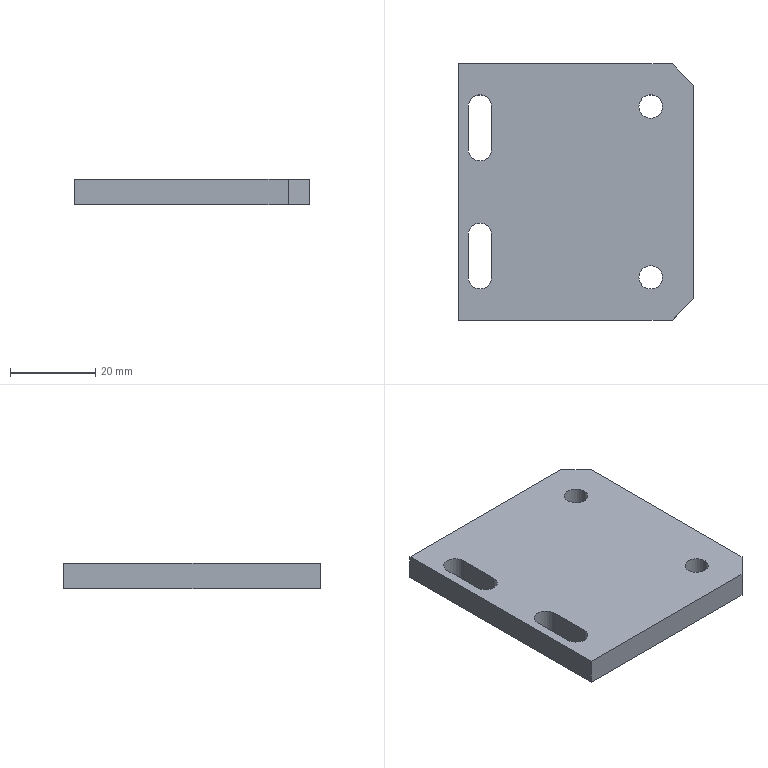Part | STEP file | 0232_206_Plate | 1 solid | 20 faces | box 55 x 60 x 6 mm | volume 18420 mm3 | plane 12 | cylinder 8 | commonest cylinder face diameters 5.5 x8
STEP:
#1=CARTESIAN_POINT('',(0.,0.,0.));
#2=DIRECTION('',(0.,0.,1.));
#3=DIRECTION('',(1.,0.,0.));
#4=AXIS2_PLACEMENT_3D('',#1,#2,#3);
#5=CARTESIAN_POINT('',(-7.25,-20.,0.));
#6=VERTEX_POINT('',#5);
#7=CARTESIAN_POINT('',(-7.25,-20.,6.));
#8=VERTEX_POINT('',#7);
#9=CARTESIAN_POINT('',(-7.25,-20.,6.));
#10=DIRECTION('',(0.,0.,1.));
#11=VECTOR('',#10,1.);
#12=LINE('',#9,#11);
#13=CARTESIAN_POINT('',(-10.,-20.,6.));
#14=DIRECTION('',(0.,0.,1.));
#15=DIRECTION('',(1.,0.,0.));
#16=AXIS2_PLACEMENT_3D('',#13,#14,#15);
#17=CYLINDRICAL_SURFACE('',#16,2.75);
#18=CARTESIAN_POINT('',(6.283,0.));
#19=DIRECTION('',(0.,1.));
#20=VECTOR('',#19,1.);
#21=LINE('',#18,#20);
#22=(GEOMETRIC_REPRESENTATION_CONTEXT(2)PARAMETRIC_REPRESENTATION_CONTEXT()REPRESENTATION_CONTEXT('',''));
#23=DEFINITIONAL_REPRESENTATION('',(#21),#22);
#24=PCURVE('',#17,#23);
#25=CARTESIAN_POINT('',(-10.,-20.,6.));
#26=DIRECTION('',(0.,0.,1.));
#27=DIRECTION('',(1.,0.,0.));
#28=AXIS2_PLACEMENT_3D('',#25,#26,#27);
#29=CYLINDRICAL_SURFACE('',#28,2.75);
#30=CARTESIAN_POINT('',(0.,0.));
#31=DIRECTION('',(0.,1.));
#32=VECTOR('',#31,1.);
#33=LINE('',#30,#32);
#34=(GEOMETRIC_REPRESENTATION_CONTEXT(2)PARAMETRIC_REPRESENTATION_CONTEXT()REPRESENTATION_CONTEXT('',''));
#35=DEFINITIONAL_REPRESENTATION('',(#33),#34);
#36=PCURVE('',#29,#35);
#37=SURFACE_CURVE('',#12,(#24,#36),.PCURVE_S1.);
#38=EDGE_CURVE('',#6,#8,#37,.T.);
#39=ORIENTED_EDGE('',*,*,#38,.T.);
#40=CARTESIAN_POINT('',(-12.75,-20.,6.));
#41=VERTEX_POINT('',#40);
#42=CARTESIAN_POINT('',(-10.,-20.,6.));
#43=DIRECTION('',(0.,0.,1.));
#44=DIRECTION('',(1.,0.,0.));
#45=AXIS2_PLACEMENT_3D('',#42,#43,#44);
#46=CIRCLE('',#45,2.75);
#47=CARTESIAN_POINT('',(0.,0.));
#48=DIRECTION('',(1.,0.));
#49=VECTOR('',#48,1.);
#50=LINE('',#47,#49);
#51=(GEOMETRIC_REPRESENTATION_CONTEXT(2)PARAMETRIC_REPRESENTATION_CONTEXT()REPRESENTATION_CONTEXT('',''));
#52=DEFINITIONAL_REPRESENTATION('',(#50),#51);
#53=PCURVE('',#17,#52);
#54=CARTESIAN_POINT('',(-55.,-30.,6.));
#55=DIRECTION('',(0.,0.,1.));
#56=DIRECTION('',(1.,0.,0.));
#57=AXIS2_PLACEMENT_3D('',#54,#55,#56);
#58=PLANE('',#57);
#59=CARTESIAN_POINT('',(45.,10.));
#60=DIRECTION('',(1.,0.));
#61=AXIS2_PLACEMENT_2D('',#59,#60);
#62=CIRCLE('',#61,2.75);
#63=(GEOMETRIC_REPRESENTATION_CONTEXT(2)PARAMETRIC_REPRESENTATION_CONTEXT()REPRESENTATION_CONTEXT('',''));
#64=DEFINITIONAL_REPRESENTATION('',(#62),#63);
#65=PCURVE('',#58,#64);
#66=SURFACE_CURVE('',#46,(#53,#65),.PCURVE_S1.);
#67=EDGE_CURVE('',#41,#8,#66,.T.);
#68=ORIENTED_EDGE('',*,*,#67,.F.);
#69=CARTESIAN_POINT('',(-12.75,-20.,0.));
#70=VERTEX_POINT('',#69);
#71=CARTESIAN_POINT('',(-12.75,-20.,6.));
#72=DIRECTION('',(0.,0.,1.));
#73=VECTOR('',#72,1.);
#74=LINE('',#71,#73);
#75=CARTESIAN_POINT('',(3.142,0.));
#76=DIRECTION('',(0.,1.));
#77=VECTOR('',#76,1.);
#78=LINE('',#75,#77);
#79=(GEOMETRIC_REPRESENTATION_CONTEXT(2)PARAMETRIC_REPRESENTATION_CONTEXT()REPRESENTATION_CONTEXT('',''));
#80=DEFINITIONAL_REPRESENTATION('',(#78),#79);
#81=PCURVE('',#17,#80);
#82=CARTESIAN_POINT('',(3.142,0.));
#83=DIRECTION('',(0.,1.));
#84=VECTOR('',#83,1.);
#85=LINE('',#82,#84);
#86=(GEOMETRIC_REPRESENTATION_CONTEXT(2)PARAMETRIC_REPRESENTATION_CONTEXT()REPRESENTATION_CONTEXT('',''));
#87=DEFINITIONAL_REPRESENTATION('',(#85),#86);
#88=PCURVE('',#29,#87);
#89=SURFACE_CURVE('',#74,(#81,#88),.PCURVE_S1.);
#90=EDGE_CURVE('',#70,#41,#89,.T.);
#91=ORIENTED_EDGE('',*,*,#90,.F.);
#92=CARTESIAN_POINT('',(-10.,-20.,0.));
#93=DIRECTION('',(0.,0.,1.));
#94=DIRECTION('',(1.,0.,0.));
#95=AXIS2_PLACEMENT_3D('',#92,#93,#94);
#96=CIRCLE('',#95,2.75);
#97=CARTESIAN_POINT('',(0.,-6.));
#98=DIRECTION('',(1.,0.));
#99=VECTOR('',#98,1.);
#100=LINE('',#97,#99);
#101=(GEOMETRIC_REPRESENTATION_CONTEXT(2)PARAMETRIC_REPRESENTATION_CONTEXT()REPRESENTATION_CONTEXT('',''));
#102=DEFINITIONAL_REPRESENTATION('',(#100),#101);
#103=PCURVE('',#17,#102);
#104=CARTESIAN_POINT('',(-55.,-30.,0.));
#105=DIRECTION('',(0.,0.,1.));
#106=DIRECTION('',(1.,0.,0.));
#107=AXIS2_PLACEMENT_3D('',#104,#105,#106);
#108=PLANE('',#107);
#109=CARTESIAN_POINT('',(45.,10.));
#110=DIRECTION('',(1.,0.));
#111=AXIS2_PLACEMENT_2D('',#109,#110);
#112=CIRCLE('',#111,2.75);
#113=(GEOMETRIC_REPRESENTATION_CONTEXT(2)PARAMETRIC_REPRESENTATION_CONTEXT()REPRESENTATION_CONTEXT('',''));
#114=DEFINITIONAL_REPRESENTATION('',(#112),#113);
#115=PCURVE('',#108,#114);
#116=SURFACE_CURVE('',#96,(#103,#115),.PCURVE_S1.);
#117=EDGE_CURVE('',#70,#6,#116,.T.);
#118=ORIENTED_EDGE('',*,*,#117,.T.);
#119=EDGE_LOOP('',(#39,#68,#91,#118));
#120=FACE_BOUND('',#119,.F.);
#121=ADVANCED_FACE('',(#120),#17,.F.);
#122=CARTESIAN_POINT('',(-7.25,20.,0.));
#123=VERTEX_POINT('',#122);
#124=CARTESIAN_POINT('',(-7.25,20.,6.));
#125=VERTEX_POINT('',#124);
#126=CARTESIAN_POINT('',(-7.25,20.,6.));
#127=DIRECTION('',(0.,0.,1.));
#128=VECTOR('',#127,1.);
#129=LINE('',#126,#128);
#130=CARTESIAN_POINT('',(-10.,20.,6.));
#131=DIRECTION('',(0.,0.,1.));
#132=DIRECTION('',(1.,0.,0.));
#133=AXIS2_PLACEMENT_3D('',#130,#131,#132);
#134=CYLINDRICAL_SURFACE('',#133,2.75);
#135=CARTESIAN_POINT('',(6.283,0.));
#136=DIRECTION('',(0.,1.));
#137=VECTOR('',#136,1.);
#138=LINE('',#135,#137);
#139=(GEOMETRIC_REPRESENTATION_CONTEXT(2)PARAMETRIC_REPRESENTATION_CONTEXT()REPRESENTATION_CONTEXT('',''));
#140=DEFINITIONAL_REPRESENTATION('',(#138),#139);
#141=PCURVE('',#134,#140);
#142=CARTESIAN_POINT('',(-10.,20.,6.));
#143=DIRECTION('',(0.,0.,1.));
#144=DIRECTION('',(1.,0.,0.));
#145=AXIS2_PLACEMENT_3D('',#142,#143,#144);
#146=CYLINDRICAL_SURFACE('',#145,2.75);
#147=CARTESIAN_POINT('',(0.,0.));
#148=DIRECTION('',(0.,1.));
#149=VECTOR('',#148,1.);
#150=LINE('',#147,#149);
#151=(GEOMETRIC_REPRESENTATION_CONTEXT(2)PARAMETRIC_REPRESENTATION_CONTEXT()REPRESENTATION_CONTEXT('',''));
#152=DEFINITIONAL_REPRESENTATION('',(#150),#151);
#153=PCURVE('',#146,#152);
#154=SURFACE_CURVE('',#129,(#141,#153),.PCURVE_S1.);
#155=EDGE_CURVE('',#123,#125,#154,.T.);
#156=ORIENTED_EDGE('',*,*,#155,.T.);
#157=CARTESIAN_POINT('',(-12.75,20.,6.));
#158=VERTEX_POINT('',#157);
#159=CARTESIAN_POINT('',(-10.,20.,6.));
#160=DIRECTION('',(0.,0.,1.));
#161=DIRECTION('',(1.,0.,0.));
#162=AXIS2_PLACEMENT_3D('',#159,#160,#161);
#163=CIRCLE('',#162,2.75);
#164=CARTESIAN_POINT('',(0.,0.));
#165=DIRECTION('',(1.,0.));
#166=VECTOR('',#165,1.);
#167=LINE('',#164,#166);
#168=(GEOMETRIC_REPRESENTATION_CONTEXT(2)PARAMETRIC_REPRESENTATION_CONTEXT()REPRESENTATION_CONTEXT('',''));
#169=DEFINITIONAL_REPRESENTATION('',(#167),#168);
#170=PCURVE('',#134,#169);
#171=CARTESIAN_POINT('',(45.,50.));
#172=DIRECTION('',(1.,0.));
#173=AXIS2_PLACEMENT_2D('',#171,#172);
#174=CIRCLE('',#173,2.75);
#175=(GEOMETRIC_REPRESENTATION_CONTEXT(2)PARAMETRIC_REPRESENTATION_CONTEXT()REPRESENTATION_CONTEXT('',''));
#176=DEFINITIONAL_REPRESENTATION('',(#174),#175);
#177=PCURVE('',#58,#176);
#178=SURFACE_CURVE('',#163,(#170,#177),.PCURVE_S1.);
#179=EDGE_CURVE('',#158,#125,#178,.T.);
#180=ORIENTED_EDGE('',*,*,#179,.F.);
#181=CARTESIAN_POINT('',(-12.75,20.,0.));
#182=VERTEX_POINT('',#181);
#183=CARTESIAN_POINT('',(-12.75,20.,6.));
#184=DIRECTION('',(0.,0.,1.));
#185=VECTOR('',#184,1.);
#186=LINE('',#183,#185);
#187=CARTESIAN_POINT('',(3.142,0.));
#188=DIRECTION('',(0.,1.));
#189=VECTOR('',#188,1.);
#190=LINE('',#187,#189);
#191=(GEOMETRIC_REPRESENTATION_CONTEXT(2)PARAMETRIC_REPRESENTATION_CONTEXT()REPRESENTATION_CONTEXT('',''));
#192=DEFINITIONAL_REPRESENTATION('',(#190),#191);
#193=PCURVE('',#134,#192);
#194=CARTESIAN_POINT('',(3.142,0.));
#195=DIRECTION('',(0.,1.));
#196=VECTOR('',#195,1.);
#197=LINE('',#194,#196);
#198=(GEOMETRIC_REPRESENTATION_CONTEXT(2)PARAMETRIC_REPRESENTATION_CONTEXT()REPRESENTATION_CONTEXT('',''));
#199=DEFINITIONAL_REPRESENTATION('',(#197),#198);
#200=PCURVE('',#146,#199);
#201=SURFACE_CURVE('',#186,(#193,#200),.PCURVE_S1.);
#202=EDGE_CURVE('',#182,#158,#201,.T.);
#203=ORIENTED_EDGE('',*,*,#202,.F.);
#204=CARTESIAN_POINT('',(-10.,20.,0.));
#205=DIRECTION('',(0.,0.,1.));
#206=DIRECTION('',(1.,0.,0.));
#207=AXIS2_PLACEMENT_3D('',#204,#205,#206);
#208=CIRCLE('',#207,2.75);
#209=CARTESIAN_POINT('',(0.,-6.));
#210=DIRECTION('',(1.,0.));
#211=VECTOR('',#210,1.);
#212=LINE('',#209,#211);
#213=(GEOMETRIC_REPRESENTATION_CONTEXT(2)PARAMETRIC_REPRESENTATION_CONTEXT()REPRESENTATION_CONTEXT('',''));
#214=DEFINITIONAL_REPRESENTATION('',(#212),#213);
#215=PCURVE('',#134,#214);
#216=CARTESIAN_POINT('',(45.,50.));
#217=DIRECTION('',(1.,0.));
#218=AXIS2_PLACEMENT_2D('',#216,#217);
#219=CIRCLE('',#218,2.75);
#220=(GEOMETRIC_REPRESENTATION_CONTEXT(2)PARAMETRIC_REPRESENTATION_CONTEXT()REPRESENTATION_CONTEXT('',''));
#221=DEFINITIONAL_REPRESENTATION('',(#219),#220);
#222=PCURVE('',#108,#221);
#223=SURFACE_CURVE('',#208,(#215,#222),.PCURVE_S1.);
#224=EDGE_CURVE('',#182,#123,#223,.T.);
#225=ORIENTED_EDGE('',*,*,#224,.T.);
#226=EDGE_LOOP('',(#156,#180,#203,#225));
#227=FACE_BOUND('',#226,.F.);
#228=ADVANCED_FACE('',(#227),#134,.F.);
#229=CARTESIAN_POINT('',(-55.,30.,0.));
#230=VERTEX_POINT('',#229);
#231=CARTESIAN_POINT('',(-55.,-30.,0.));
#232=VERTEX_POINT('',#231);
#233=CARTESIAN_POINT('',(-55.,30.,0.));
#234=DIRECTION('',(0.,-1.,0.));
#235=VECTOR('',#234,1.);
#236=LINE('',#233,#235);
#237=CARTESIAN_POINT('',(-55.,30.,6.));
#238=DIRECTION('',(1.,0.,0.));
#239=DIRECTION('',(0.,0.,-1.));
#240=AXIS2_PLACEMENT_3D('',#237,#238,#239);
#241=PLANE('',#240);
#242=CARTESIAN_POINT('',(6.,0.));
#243=DIRECTION('',(0.,-1.));
#244=VECTOR('',#243,1.);
#245=LINE('',#242,#244);
#246=(GEOMETRIC_REPRESENTATION_CONTEXT(2)PARAMETRIC_REPRESENTATION_CONTEXT()REPRESENTATION_CONTEXT('',''));
#247=DEFINITIONAL_REPRESENTATION('',(#245),#246);
#248=PCURVE('',#241,#247);
#249=CARTESIAN_POINT('',(0.,60.));
#250=DIRECTION('',(0.,-1.));
#251=VECTOR('',#250,1.);
#252=LINE('',#249,#251);
#253=(GEOMETRIC_REPRESENTATION_CONTEXT(2)PARAMETRIC_REPRESENTATION_CONTEXT()REPRESENTATION_CONTEXT('',''));
#254=DEFINITIONAL_REPRESENTATION('',(#252),#253);
#255=PCURVE('',#108,#254);
#256=SURFACE_CURVE('',#236,(#248,#255),.PCURVE_S1.);
#257=EDGE_CURVE('',#230,#232,#256,.T.);
#258=ORIENTED_EDGE('',*,*,#257,.T.);
#259=CARTESIAN_POINT('',(-55.,-30.,6.));
#260=VERTEX_POINT('',#259);
#261=CARTESIAN_POINT('',(-55.,-30.,6.));
#262=DIRECTION('',(0.,0.,-1.));
#263=VECTOR('',#262,1.);
#264=LINE('',#261,#263);
#265=CARTESIAN_POINT('',(0.,-60.));
#266=DIRECTION('',(1.,0.));
#267=VECTOR('',#266,1.);
#268=LINE('',#265,#267);
#269=(GEOMETRIC_REPRESENTATION_CONTEXT(2)PARAMETRIC_REPRESENTATION_CONTEXT()REPRESENTATION_CONTEXT('',''));
#270=DEFINITIONAL_REPRESENTATION('',(#268),#269);
#271=PCURVE('',#241,#270);
#272=CARTESIAN_POINT('',(-55.,-30.,6.));
#273=DIRECTION('',(0.,1.,0.));
#274=DIRECTION('',(0.,0.,1.));
#275=AXIS2_PLACEMENT_3D('',#272,#273,#274);
#276=PLANE('',#275);
#277=CARTESIAN_POINT('',(0.,0.));
#278=DIRECTION('',(-1.,0.));
#279=VECTOR('',#278,1.);
#280=LINE('',#277,#279);
#281=(GEOMETRIC_REPRESENTATION_CONTEXT(2)PARAMETRIC_REPRESENTATION_CONTEXT()REPRESENTATION_CONTEXT('',''));
#282=DEFINITIONAL_REPRESENTATION('',(#280),#281);
#283=PCURVE('',#276,#282);
#284=SURFACE_CURVE('',#264,(#271,#283),.PCURVE_S1.);
#285=EDGE_CURVE('',#260,#232,#284,.T.);
#286=ORIENTED_EDGE('',*,*,#285,.F.);
#287=CARTESIAN_POINT('',(-55.,30.,6.));
#288=VERTEX_POINT('',#287);
#289=CARTESIAN_POINT('',(-55.,30.,6.));
#290=DIRECTION('',(0.,-1.,0.));
#291=VECTOR('',#290,1.);
#292=LINE('',#289,#291);
#293=CARTESIAN_POINT('',(0.,0.));
#294=DIRECTION('',(0.,-1.));
#295=VECTOR('',#294,1.);
#296=LINE('',#293,#295);
#297=(GEOMETRIC_REPRESENTATION_CONTEXT(2)PARAMETRIC_REPRESENTATION_CONTEXT()REPRESENTATION_CONTEXT('',''));
#298=DEFINITIONAL_REPRESENTATION('',(#296),#297);
#299=PCURVE('',#241,#298);
#300=CARTESIAN_POINT('',(0.,60.));
#301=DIRECTION('',(0.,-1.));
#302=VECTOR('',#301,1.);
#303=LINE('',#300,#302);
#304=(GEOMETRIC_REPRESENTATION_CONTEXT(2)PARAMETRIC_REPRESENTATION_CONTEXT()REPRESENTATION_CONTEXT('',''));
#305=DEFINITIONAL_REPRESENTATION('',(#303),#304);
#306=PCURVE('',#58,#305);
#307=SURFACE_CURVE('',#292,(#299,#306),.PCURVE_S1.);
#308=EDGE_CURVE('',#288,#260,#307,.T.);
#309=ORIENTED_EDGE('',*,*,#308,.F.);
#310=CARTESIAN_POINT('',(-55.,30.,6.));
#311=DIRECTION('',(0.,0.,-1.));
#312=VECTOR('',#311,1.);
#313=LINE('',#310,#312);
#314=CARTESIAN_POINT('',(0.,0.));
#315=DIRECTION('',(1.,0.));
#316=VECTOR('',#315,1.);
#317=LINE('',#314,#316);
#318=(GEOMETRIC_REPRESENTATION_CONTEXT(2)PARAMETRIC_REPRESENTATION_CONTEXT()REPRESENTATION_CONTEXT('',''));
#319=DEFINITIONAL_REPRESENTATION('',(#317),#318);
#320=PCURVE('',#241,#319);
#321=CARTESIAN_POINT('',(-55.,30.,6.));
#322=DIRECTION('',(0.,-1.,0.));
#323=DIRECTION('',(0.,0.,-1.));
#324=AXIS2_PLACEMENT_3D('',#321,#322,#323);
#325=PLANE('',#324);
#326=CARTESIAN_POINT('',(0.,0.));
#327=DIRECTION('',(1.,0.));
#328=VECTOR('',#327,1.);
#329=LINE('',#326,#328);
#330=(GEOMETRIC_REPRESENTATION_CONTEXT(2)PARAMETRIC_REPRESENTATION_CONTEXT()REPRESENTATION_CONTEXT('',''));
#331=DEFINITIONAL_REPRESENTATION('',(#329),#330);
#332=PCURVE('',#325,#331);
#333=SURFACE_CURVE('',#313,(#320,#332),.PCURVE_S1.);
#334=EDGE_CURVE('',#288,#230,#333,.T.);
#335=ORIENTED_EDGE('',*,*,#334,.T.);
#336=EDGE_LOOP('',(#258,#286,#309,#335));
#337=FACE_BOUND('',#336,.T.);
#338=ADVANCED_FACE('',(#337),#241,.F.);
#339=CARTESIAN_POINT('',(-5.,-30.,0.));
#340=VERTEX_POINT('',#339);
#341=CARTESIAN_POINT('',(-55.,-30.,0.));
#342=DIRECTION('',(1.,0.,0.));
#343=VECTOR('',#342,1.);
#344=LINE('',#341,#343);
#345=CARTESIAN_POINT('',(-6.,0.));
#346=DIRECTION('',(0.,1.));
#347=VECTOR('',#346,1.);
#348=LINE('',#345,#347);
#349=(GEOMETRIC_REPRESENTATION_CONTEXT(2)PARAMETRIC_REPRESENTATION_CONTEXT()REPRESENTATION_CONTEXT('',''));
#350=DEFINITIONAL_REPRESENTATION('',(#348),#349);
#351=PCURVE('',#276,#350);
#352=CARTESIAN_POINT('',(0.,0.));
#353=DIRECTION('',(1.,0.));
#354=VECTOR('',#353,1.);
#355=LINE('',#352,#354);
#356=(GEOMETRIC_REPRESENTATION_CONTEXT(2)PARAMETRIC_REPRESENTATION_CONTEXT()REPRESENTATION_CONTEXT('',''));
#357=DEFINITIONAL_REPRESENTATION('',(#355),#356);
#358=PCURVE('',#108,#357);
#359=SURFACE_CURVE('',#344,(#351,#358),.PCURVE_S1.);
#360=EDGE_CURVE('',#232,#340,#359,.T.);
#361=ORIENTED_EDGE('',*,*,#360,.T.);
#362=CARTESIAN_POINT('',(-5.,-30.,6.));
#363=VERTEX_POINT('',#362);
#364=CARTESIAN_POINT('',(-5.,-30.,6.));
#365=DIRECTION('',(0.,0.,1.));
#366=VECTOR('',#365,1.);
#367=LINE('',#364,#366);
#368=CARTESIAN_POINT('',(0.,50.));
#369=DIRECTION('',(1.,0.));
#370=VECTOR('',#369,1.);
#371=LINE('',#368,#370);
#372=(GEOMETRIC_REPRESENTATION_CONTEXT(2)PARAMETRIC_REPRESENTATION_CONTEXT()REPRESENTATION_CONTEXT('',''));
#373=DEFINITIONAL_REPRESENTATION('',(#371),#372);
#374=PCURVE('',#276,#373);
#375=CARTESIAN_POINT('',(0.,-25.,6.));
#376=DIRECTION('',(-0.7071,0.7071,0.));
#377=DIRECTION('',(-0.7071,-0.7071,0.));
#378=AXIS2_PLACEMENT_3D('',#375,#376,#377);
#379=PLANE('',#378);
#380=CARTESIAN_POINT('',(7.071,0.));
#381=DIRECTION('',(0.,1.));
#382=VECTOR('',#381,1.);
#383=LINE('',#380,#382);
#384=(GEOMETRIC_REPRESENTATION_CONTEXT(2)PARAMETRIC_REPRESENTATION_CONTEXT()REPRESENTATION_CONTEXT('',''));
#385=DEFINITIONAL_REPRESENTATION('',(#383),#384);
#386=PCURVE('',#379,#385);
#387=SURFACE_CURVE('',#367,(#374,#386),.PCURVE_S1.);
#388=EDGE_CURVE('',#340,#363,#387,.T.);
#389=ORIENTED_EDGE('',*,*,#388,.T.);
#390=CARTESIAN_POINT('',(-55.,-30.,6.));
#391=DIRECTION('',(1.,0.,0.));
#392=VECTOR('',#391,1.);
#393=LINE('',#390,#392);
#394=CARTESIAN_POINT('',(0.,0.));
#395=DIRECTION('',(0.,1.));
#396=VECTOR('',#395,1.);
#397=LINE('',#394,#396);
#398=(GEOMETRIC_REPRESENTATION_CONTEXT(2)PARAMETRIC_REPRESENTATION_CONTEXT()REPRESENTATION_CONTEXT('',''));
#399=DEFINITIONAL_REPRESENTATION('',(#397),#398);
#400=PCURVE('',#276,#399);
#401=CARTESIAN_POINT('',(0.,0.));
#402=DIRECTION('',(1.,0.));
#403=VECTOR('',#402,1.);
#404=LINE('',#401,#403);
#405=(GEOMETRIC_REPRESENTATION_CONTEXT(2)PARAMETRIC_REPRESENTATION_CONTEXT()REPRESENTATION_CONTEXT('',''));
#406=DEFINITIONAL_REPRESENTATION('',(#404),#405);
#407=PCURVE('',#58,#406);
#408=SURFACE_CURVE('',#393,(#400,#407),.PCURVE_S1.);
#409=EDGE_CURVE('',#260,#363,#408,.T.);
#410=ORIENTED_EDGE('',*,*,#409,.F.);
#411=ORIENTED_EDGE('',*,*,#285,.T.);
#412=EDGE_LOOP('',(#361,#389,#410,#411));
#413=FACE_BOUND('',#412,.T.);
#414=ADVANCED_FACE('',(#413),#276,.F.);
#415=CARTESIAN_POINT('',(0.,-25.,6.));
#416=VERTEX_POINT('',#415);
#417=CARTESIAN_POINT('',(0.,25.,6.));
#418=VERTEX_POINT('',#417);
#419=CARTESIAN_POINT('',(0.,30.,6.));
#420=DIRECTION('',(0.,1.,0.));
#421=VECTOR('',#420,1.);
#422=LINE('',#419,#421);
#423=CARTESIAN_POINT('',(0.,30.,6.));
#424=DIRECTION('',(-1.,0.,0.));
#425=DIRECTION('',(0.,0.,1.));
#426=AXIS2_PLACEMENT_3D('',#423,#424,#425);
#427=PLANE('',#426);
#428=CARTESIAN_POINT('',(0.,0.));
#429=DIRECTION('',(0.,1.));
#430=VECTOR('',#429,1.);
#431=LINE('',#428,#430);
#432=(GEOMETRIC_REPRESENTATION_CONTEXT(2)PARAMETRIC_REPRESENTATION_CONTEXT()REPRESENTATION_CONTEXT('',''));
#433=DEFINITIONAL_REPRESENTATION('',(#431),#432);
#434=PCURVE('',#427,#433);
#435=CARTESIAN_POINT('',(55.,60.));
#436=DIRECTION('',(0.,1.));
#437=VECTOR('',#436,1.);
#438=LINE('',#435,#437);
#439=(GEOMETRIC_REPRESENTATION_CONTEXT(2)PARAMETRIC_REPRESENTATION_CONTEXT()REPRESENTATION_CONTEXT('',''));
#440=DEFINITIONAL_REPRESENTATION('',(#438),#439);
#441=PCURVE('',#58,#440);
#442=SURFACE_CURVE('',#422,(#434,#441),.PCURVE_S1.);
#443=EDGE_CURVE('',#416,#418,#442,.T.);
#444=ORIENTED_EDGE('',*,*,#443,.F.);
#445=CARTESIAN_POINT('',(0.,-25.,0.));
#446=VERTEX_POINT('',#445);
#447=CARTESIAN_POINT('',(0.,-25.,6.));
#448=DIRECTION('',(0.,0.,-1.));
#449=VECTOR('',#448,1.);
#450=LINE('',#447,#449);
#451=CARTESIAN_POINT('',(0.,-55.));
#452=DIRECTION('',(-1.,0.));
#453=VECTOR('',#452,1.);
#454=LINE('',#451,#453);
#455=(GEOMETRIC_REPRESENTATION_CONTEXT(2)PARAMETRIC_REPRESENTATION_CONTEXT()REPRESENTATION_CONTEXT('',''));
#456=DEFINITIONAL_REPRESENTATION('',(#454),#455);
#457=PCURVE('',#427,#456);
#458=CARTESIAN_POINT('',(0.,0.));
#459=DIRECTION('',(0.,-1.));
#460=VECTOR('',#459,1.);
#461=LINE('',#458,#460);
#462=(GEOMETRIC_REPRESENTATION_CONTEXT(2)PARAMETRIC_REPRESENTATION_CONTEXT()REPRESENTATION_CONTEXT('',''));
#463=DEFINITIONAL_REPRESENTATION('',(#461),#462);
#464=PCURVE('',#379,#463);
#465=SURFACE_CURVE('',#450,(#457,#464),.PCURVE_S1.);
#466=EDGE_CURVE('',#416,#446,#465,.T.);
#467=ORIENTED_EDGE('',*,*,#466,.T.);
#468=CARTESIAN_POINT('',(0.,25.,0.));
#469=VERTEX_POINT('',#468);
#470=CARTESIAN_POINT('',(0.,30.,0.));
#471=DIRECTION('',(0.,1.,0.));
#472=VECTOR('',#471,1.);
#473=LINE('',#470,#472);
#474=CARTESIAN_POINT('',(-6.,0.));
#475=DIRECTION('',(0.,1.));
#476=VECTOR('',#475,1.);
#477=LINE('',#474,#476);
#478=(GEOMETRIC_REPRESENTATION_CONTEXT(2)PARAMETRIC_REPRESENTATION_CONTEXT()REPRESENTATION_CONTEXT('',''));
#479=DEFINITIONAL_REPRESENTATION('',(#477),#478);
#480=PCURVE('',#427,#479);
#481=CARTESIAN_POINT('',(55.,60.));
#482=DIRECTION('',(0.,1.));
#483=VECTOR('',#482,1.);
#484=LINE('',#481,#483);
#485=(GEOMETRIC_REPRESENTATION_CONTEXT(2)PARAMETRIC_REPRESENTATION_CONTEXT()REPRESENTATION_CONTEXT('',''));
#486=DEFINITIONAL_REPRESENTATION('',(#484),#485);
#487=PCURVE('',#108,#486);
#488=SURFACE_CURVE('',#473,(#480,#487),.PCURVE_S1.);
#489=EDGE_CURVE('',#446,#469,#488,.T.);
#490=ORIENTED_EDGE('',*,*,#489,.T.);
#491=CARTESIAN_POINT('',(0.,25.,6.));
#492=DIRECTION('',(0.,0.,1.));
#493=VECTOR('',#492,1.);
#494=LINE('',#491,#493);
#495=CARTESIAN_POINT('',(0.,-5.));
#496=DIRECTION('',(1.,0.));
#497=VECTOR('',#496,1.);
#498=LINE('',#495,#497);
#499=(GEOMETRIC_REPRESENTATION_CONTEXT(2)PARAMETRIC_REPRESENTATION_CONTEXT()REPRESENTATION_CONTEXT('',''));
#500=DEFINITIONAL_REPRESENTATION('',(#498),#499);
#501=PCURVE('',#427,#500);
#502=CARTESIAN_POINT('',(-5.,30.,6.));
#503=DIRECTION('',(-0.7071,-0.7071,0.));
#504=DIRECTION('',(0.7071,-0.7071,0.));
#505=AXIS2_PLACEMENT_3D('',#502,#503,#504);
#506=PLANE('',#505);
#507=CARTESIAN_POINT('',(7.071,0.));
#508=DIRECTION('',(0.,1.));
#509=VECTOR('',#508,1.);
#510=LINE('',#507,#509);
#511=(GEOMETRIC_REPRESENTATION_CONTEXT(2)PARAMETRIC_REPRESENTATION_CONTEXT()REPRESENTATION_CONTEXT('',''));
#512=DEFINITIONAL_REPRESENTATION('',(#510),#511);
#513=PCURVE('',#506,#512);
#514=SURFACE_CURVE('',#494,(#501,#513),.PCURVE_S1.);
#515=EDGE_CURVE('',#469,#418,#514,.T.);
#516=ORIENTED_EDGE('',*,*,#515,.T.);
#517=EDGE_LOOP('',(#444,#467,#490,#516));
#518=FACE_BOUND('',#517,.T.);
#519=ADVANCED_FACE('',(#518),#427,.F.);
#520=CARTESIAN_POINT('',(-5.,30.,6.));
#521=VERTEX_POINT('',#520);
#522=CARTESIAN_POINT('',(-55.,30.,6.));
#523=DIRECTION('',(-1.,0.,0.));
#524=VECTOR('',#523,1.);
#525=LINE('',#522,#524);
#526=CARTESIAN_POINT('',(0.,0.));
#527=DIRECTION('',(0.,-1.));
#528=VECTOR('',#527,1.);
#529=LINE('',#526,#528);
#530=(GEOMETRIC_REPRESENTATION_CONTEXT(2)PARAMETRIC_REPRESENTATION_CONTEXT()REPRESENTATION_CONTEXT('',''));
#531=DEFINITIONAL_REPRESENTATION('',(#529),#530);
#532=PCURVE('',#325,#531);
#533=CARTESIAN_POINT('',(0.,60.));
#534=DIRECTION('',(-1.,0.));
#535=VECTOR('',#534,1.);
#536=LINE('',#533,#535);
#537=(GEOMETRIC_REPRESENTATION_CONTEXT(2)PARAMETRIC_REPRESENTATION_CONTEXT()REPRESENTATION_CONTEXT('',''));
#538=DEFINITIONAL_REPRESENTATION('',(#536),#537);
#539=PCURVE('',#58,#538);
#540=SURFACE_CURVE('',#525,(#532,#539),.PCURVE_S1.);
#541=EDGE_CURVE('',#521,#288,#540,.T.);
#542=ORIENTED_EDGE('',*,*,#541,.F.);
#543=CARTESIAN_POINT('',(-5.,30.,0.));
#544=VERTEX_POINT('',#543);
#545=CARTESIAN_POINT('',(-5.,30.,6.));
#546=DIRECTION('',(0.,0.,-1.));
#547=VECTOR('',#546,1.);
#548=LINE('',#545,#547);
#549=CARTESIAN_POINT('',(0.,50.));
#550=DIRECTION('',(1.,0.));
#551=VECTOR('',#550,1.);
#552=LINE('',#549,#551);
#553=(GEOMETRIC_REPRESENTATION_CONTEXT(2)PARAMETRIC_REPRESENTATION_CONTEXT()REPRESENTATION_CONTEXT('',''));
#554=DEFINITIONAL_REPRESENTATION('',(#552),#553);
#555=PCURVE('',#325,#554);
#556=CARTESIAN_POINT('',(0.,0.));
#557=DIRECTION('',(0.,-1.));
#558=VECTOR('',#557,1.);
#559=LINE('',#556,#558);
#560=(GEOMETRIC_REPRESENTATION_CONTEXT(2)PARAMETRIC_REPRESENTATION_CONTEXT()REPRESENTATION_CONTEXT('',''));
#561=DEFINITIONAL_REPRESENTATION('',(#559),#560);
#562=PCURVE('',#506,#561);
#563=SURFACE_CURVE('',#548,(#555,#562),.PCURVE_S1.);
#564=EDGE_CURVE('',#521,#544,#563,.T.);
#565=ORIENTED_EDGE('',*,*,#564,.T.);
#566=CARTESIAN_POINT('',(-55.,30.,0.));
#567=DIRECTION('',(-1.,0.,0.));
#568=VECTOR('',#567,1.);
#569=LINE('',#566,#568);
#570=CARTESIAN_POINT('',(6.,0.));
#571=DIRECTION('',(0.,-1.));
#572=VECTOR('',#571,1.);
#573=LINE('',#570,#572);
#574=(GEOMETRIC_REPRESENTATION_CONTEXT(2)PARAMETRIC_REPRESENTATION_CONTEXT()REPRESENTATION_CONTEXT('',''));
#575=DEFINITIONAL_REPRESENTATION('',(#573),#574);
#576=PCURVE('',#325,#575);
#577=CARTESIAN_POINT('',(0.,60.));
#578=DIRECTION('',(-1.,0.));
#579=VECTOR('',#578,1.);
#580=LINE('',#577,#579);
#581=(GEOMETRIC_REPRESENTATION_CONTEXT(2)PARAMETRIC_REPRESENTATION_CONTEXT()REPRESENTATION_CONTEXT('',''));
#582=DEFINITIONAL_REPRESENTATION('',(#580),#581);
#583=PCURVE('',#108,#582);
#584=SURFACE_CURVE('',#569,(#576,#583),.PCURVE_S1.);
#585=EDGE_CURVE('',#544,#230,#584,.T.);
#586=ORIENTED_EDGE('',*,*,#585,.T.);
#587=ORIENTED_EDGE('',*,*,#334,.F.);
#588=EDGE_LOOP('',(#542,#565,#586,#587));
#589=FACE_BOUND('',#588,.T.);
#590=ADVANCED_FACE('',(#589),#325,.F.);
#591=CARTESIAN_POINT('',(-10.,-20.,6.));
#592=DIRECTION('',(0.,0.,1.));
#593=DIRECTION('',(1.,0.,0.));
#594=AXIS2_PLACEMENT_3D('',#591,#592,#593);
#595=CIRCLE('',#594,2.75);
#596=CARTESIAN_POINT('',(45.,10.));
#597=DIRECTION('',(1.,0.));
#598=AXIS2_PLACEMENT_2D('',#596,#597);
#599=CIRCLE('',#598,2.75);
#600=(GEOMETRIC_REPRESENTATION_CONTEXT(2)PARAMETRIC_REPRESENTATION_CONTEXT()REPRESENTATION_CONTEXT('',''));
#601=DEFINITIONAL_REPRESENTATION('',(#599),#600);
#602=PCURVE('',#58,#601);
#603=CARTESIAN_POINT('',(0.,0.));
#604=DIRECTION('',(1.,0.));
#605=VECTOR('',#604,1.);
#606=LINE('',#603,#605);
#607=(GEOMETRIC_REPRESENTATION_CONTEXT(2)PARAMETRIC_REPRESENTATION_CONTEXT()REPRESENTATION_CONTEXT('',''));
#608=DEFINITIONAL_REPRESENTATION('',(#606),#607);
#609=PCURVE('',#29,#608);
#610=SURFACE_CURVE('',#595,(#602,#609),.PCURVE_S1.);
#611=EDGE_CURVE('',#8,#41,#610,.T.);
#612=ORIENTED_EDGE('',*,*,#611,.F.);
#613=ORIENTED_EDGE('',*,*,#67,.F.);
#614=EDGE_LOOP('',(#612,#613));
#615=FACE_BOUND('',#614,.T.);
#616=CARTESIAN_POINT('',(-10.,20.,6.));
#617=DIRECTION('',(0.,0.,1.));
#618=DIRECTION('',(1.,0.,0.));
#619=AXIS2_PLACEMENT_3D('',#616,#617,#618);
#620=CIRCLE('',#619,2.75);
#621=CARTESIAN_POINT('',(45.,50.));
#622=DIRECTION('',(1.,0.));
#623=AXIS2_PLACEMENT_2D('',#621,#622);
#624=CIRCLE('',#623,2.75);
#625=(GEOMETRIC_REPRESENTATION_CONTEXT(2)PARAMETRIC_REPRESENTATION_CONTEXT()REPRESENTATION_CONTEXT('',''));
#626=DEFINITIONAL_REPRESENTATION('',(#624),#625);
#627=PCURVE('',#58,#626);
#628=CARTESIAN_POINT('',(0.,0.));
#629=DIRECTION('',(1.,0.));
#630=VECTOR('',#629,1.);
#631=LINE('',#628,#630);
#632=(GEOMETRIC_REPRESENTATION_CONTEXT(2)PARAMETRIC_REPRESENTATION_CONTEXT()REPRESENTATION_CONTEXT('',''));
#633=DEFINITIONAL_REPRESENTATION('',(#631),#632);
#634=PCURVE('',#146,#633);
#635=SURFACE_CURVE('',#620,(#627,#634),.PCURVE_S1.);
#636=EDGE_CURVE('',#125,#158,#635,.T.);
#637=ORIENTED_EDGE('',*,*,#636,.F.);
#638=ORIENTED_EDGE('',*,*,#179,.F.);
#639=EDGE_LOOP('',(#637,#638));
#640=FACE_BOUND('',#639,.T.);
#641=CARTESIAN_POINT('',(-47.25,20.,6.));
#642=VERTEX_POINT('',#641);
#643=CARTESIAN_POINT('',(-52.75,20.,6.));
#644=VERTEX_POINT('',#643);
#645=CARTESIAN_POINT('',(-50.,20.,6.));
#646=DIRECTION('',(0.,0.,1.));
#647=DIRECTION('',(1.,0.,0.));
#648=AXIS2_PLACEMENT_3D('',#645,#646,#647);
#649=CIRCLE('',#648,2.75);
#650=CARTESIAN_POINT('',(5.,50.));
#651=DIRECTION('',(1.,0.));
#652=AXIS2_PLACEMENT_2D('',#650,#651);
#653=CIRCLE('',#652,2.75);
#654=(GEOMETRIC_REPRESENTATION_CONTEXT(2)PARAMETRIC_REPRESENTATION_CONTEXT()REPRESENTATION_CONTEXT('',''));
#655=DEFINITIONAL_REPRESENTATION('',(#653),#654);
#656=PCURVE('',#58,#655);
#657=CARTESIAN_POINT('',(-50.,20.,0.));
#658=DIRECTION('',(0.,0.,1.));
#659=DIRECTION('',(1.,0.,0.));
#660=AXIS2_PLACEMENT_3D('',#657,#658,#659);
#661=CYLINDRICAL_SURFACE('',#660,2.75);
#662=CARTESIAN_POINT('',(0.,6.));
#663=DIRECTION('',(1.,0.));
#664=VECTOR('',#663,1.);
#665=LINE('',#662,#664);
#666=(GEOMETRIC_REPRESENTATION_CONTEXT(2)PARAMETRIC_REPRESENTATION_CONTEXT()REPRESENTATION_CONTEXT('',''));
#667=DEFINITIONAL_REPRESENTATION('',(#665),#666);
#668=PCURVE('',#661,#667);
#669=SURFACE_CURVE('',#649,(#656,#668),.PCURVE_S1.);
#670=EDGE_CURVE('',#642,#644,#669,.T.);
#671=ORIENTED_EDGE('',*,*,#670,.F.);
#672=CARTESIAN_POINT('',(-47.25,10.,6.));
#673=VERTEX_POINT('',#672);
#674=CARTESIAN_POINT('',(-47.25,20.,6.));
#675=DIRECTION('',(0.,1.,0.));
#676=VECTOR('',#675,1.);
#677=LINE('',#674,#676);
#678=CARTESIAN_POINT('',(7.75,50.));
#679=DIRECTION('',(0.,1.));
#680=VECTOR('',#679,1.);
#681=LINE('',#678,#680);
#682=(GEOMETRIC_REPRESENTATION_CONTEXT(2)PARAMETRIC_REPRESENTATION_CONTEXT()REPRESENTATION_CONTEXT('',''));
#683=DEFINITIONAL_REPRESENTATION('',(#681),#682);
#684=PCURVE('',#58,#683);
#685=CARTESIAN_POINT('',(-47.25,20.,0.));
#686=DIRECTION('',(1.,0.,0.));
#687=DIRECTION('',(0.,0.,-1.));
#688=AXIS2_PLACEMENT_3D('',#685,#686,#687);
#689=PLANE('',#688);
#690=CARTESIAN_POINT('',(-6.,0.));
#691=DIRECTION('',(0.,1.));
#692=VECTOR('',#691,1.);
#693=LINE('',#690,#692);
#694=(GEOMETRIC_REPRESENTATION_CONTEXT(2)PARAMETRIC_REPRESENTATION_CONTEXT()REPRESENTATION_CONTEXT('',''));
#695=DEFINITIONAL_REPRESENTATION('',(#693),#694);
#696=PCURVE('',#689,#695);
#697=SURFACE_CURVE('',#677,(#684,#696),.PCURVE_S1.);
#698=EDGE_CURVE('',#673,#642,#697,.T.);
#699=ORIENTED_EDGE('',*,*,#698,.F.);
#700=CARTESIAN_POINT('',(-52.75,10.,6.));
#701=VERTEX_POINT('',#700);
#702=CARTESIAN_POINT('',(-50.,10.,6.));
#703=DIRECTION('',(0.,0.,1.));
#704=DIRECTION('',(1.,0.,0.));
#705=AXIS2_PLACEMENT_3D('',#702,#703,#704);
#706=CIRCLE('',#705,2.75);
#707=CARTESIAN_POINT('',(5.,40.));
#708=DIRECTION('',(1.,0.));
#709=AXIS2_PLACEMENT_2D('',#707,#708);
#710=CIRCLE('',#709,2.75);
#711=(GEOMETRIC_REPRESENTATION_CONTEXT(2)PARAMETRIC_REPRESENTATION_CONTEXT()REPRESENTATION_CONTEXT('',''));
#712=DEFINITIONAL_REPRESENTATION('',(#710),#711);
#713=PCURVE('',#58,#712);
#714=CARTESIAN_POINT('',(-50.,10.,0.));
#715=DIRECTION('',(0.,0.,1.));
#716=DIRECTION('',(1.,0.,0.));
#717=AXIS2_PLACEMENT_3D('',#714,#715,#716);
#718=CYLINDRICAL_SURFACE('',#717,2.75);
#719=CARTESIAN_POINT('',(0.,6.));
#720=DIRECTION('',(1.,0.));
#721=VECTOR('',#720,1.);
#722=LINE('',#719,#721);
#723=(GEOMETRIC_REPRESENTATION_CONTEXT(2)PARAMETRIC_REPRESENTATION_CONTEXT()REPRESENTATION_CONTEXT('',''));
#724=DEFINITIONAL_REPRESENTATION('',(#722),#723);
#725=PCURVE('',#718,#724);
#726=SURFACE_CURVE('',#706,(#713,#725),.PCURVE_S1.);
#727=EDGE_CURVE('',#701,#673,#726,.T.);
#728=ORIENTED_EDGE('',*,*,#727,.F.);
#729=CARTESIAN_POINT('',(-52.75,20.,6.));
#730=DIRECTION('',(0.,-1.,0.));
#731=VECTOR('',#730,1.);
#732=LINE('',#729,#731);
#733=CARTESIAN_POINT('',(2.25,50.));
#734=DIRECTION('',(0.,-1.));
#735=VECTOR('',#734,1.);
#736=LINE('',#733,#735);
#737=(GEOMETRIC_REPRESENTATION_CONTEXT(2)PARAMETRIC_REPRESENTATION_CONTEXT()REPRESENTATION_CONTEXT('',''));
#738=DEFINITIONAL_REPRESENTATION('',(#736),#737);
#739=PCURVE('',#58,#738);
#740=CARTESIAN_POINT('',(-52.75,20.,0.));
#741=DIRECTION('',(-1.,0.,0.));
#742=DIRECTION('',(0.,0.,1.));
#743=AXIS2_PLACEMENT_3D('',#740,#741,#742);
#744=PLANE('',#743);
#745=CARTESIAN_POINT('',(6.,0.));
#746=DIRECTION('',(0.,-1.));
#747=VECTOR('',#746,1.);
#748=LINE('',#745,#747);
#749=(GEOMETRIC_REPRESENTATION_CONTEXT(2)PARAMETRIC_REPRESENTATION_CONTEXT()REPRESENTATION_CONTEXT('',''));
#750=DEFINITIONAL_REPRESENTATION('',(#748),#749);
#751=PCURVE('',#744,#750);
#752=SURFACE_CURVE('',#732,(#739,#751),.PCURVE_S1.);
#753=EDGE_CURVE('',#644,#701,#752,.T.);
#754=ORIENTED_EDGE('',*,*,#753,.F.);
#755=EDGE_LOOP('',(#671,#699,#728,#754));
#756=FACE_BOUND('',#755,.T.);
#757=CARTESIAN_POINT('',(-52.75,-20.,6.));
#758=VERTEX_POINT('',#757);
#759=CARTESIAN_POINT('',(-47.25,-20.,6.));
#760=VERTEX_POINT('',#759);
#761=CARTESIAN_POINT('',(-50.,-20.,6.));
#762=DIRECTION('',(0.,0.,1.));
#763=DIRECTION('',(-1.,0.,0.));
#764=AXIS2_PLACEMENT_3D('',#761,#762,#763);
#765=CIRCLE('',#764,2.75);
#766=CARTESIAN_POINT('',(5.,10.));
#767=DIRECTION('',(-1.,0.));
#768=AXIS2_PLACEMENT_2D('',#766,#767);
#769=CIRCLE('',#768,2.75);
#770=(GEOMETRIC_REPRESENTATION_CONTEXT(2)PARAMETRIC_REPRESENTATION_CONTEXT()REPRESENTATION_CONTEXT('',''));
#771=DEFINITIONAL_REPRESENTATION('',(#769),#770);
#772=PCURVE('',#58,#771);
#773=CARTESIAN_POINT('',(-50.,-20.,0.));
#774=DIRECTION('',(0.,0.,1.));
#775=DIRECTION('',(1.,0.,0.));
#776=AXIS2_PLACEMENT_3D('',#773,#774,#775);
#777=CYLINDRICAL_SURFACE('',#776,2.75);
#778=CARTESIAN_POINT('',(3.142,6.));
#779=DIRECTION('',(1.,0.));
#780=VECTOR('',#779,1.);
#781=LINE('',#778,#780);
#782=(GEOMETRIC_REPRESENTATION_CONTEXT(2)PARAMETRIC_REPRESENTATION_CONTEXT()REPRESENTATION_CONTEXT('',''));
#783=DEFINITIONAL_REPRESENTATION('',(#781),#782);
#784=PCURVE('',#777,#783);
#785=SURFACE_CURVE('',#765,(#772,#784),.PCURVE_S1.);
#786=EDGE_CURVE('',#758,#760,#785,.T.);
#787=ORIENTED_EDGE('',*,*,#786,.F.);
#788=CARTESIAN_POINT('',(-52.75,-10.,6.));
#789=VERTEX_POINT('',#788);
#790=CARTESIAN_POINT('',(-52.75,-20.,6.));
#791=DIRECTION('',(0.,-1.,0.));
#792=VECTOR('',#791,1.);
#793=LINE('',#790,#792);
#794=CARTESIAN_POINT('',(2.25,10.));
#795=DIRECTION('',(0.,-1.));
#796=VECTOR('',#795,1.);
#797=LINE('',#794,#796);
#798=(GEOMETRIC_REPRESENTATION_CONTEXT(2)PARAMETRIC_REPRESENTATION_CONTEXT()REPRESENTATION_CONTEXT('',''));
#799=DEFINITIONAL_REPRESENTATION('',(#797),#798);
#800=PCURVE('',#58,#799);
#801=CARTESIAN_POINT('',(-52.75,-20.,0.));
#802=DIRECTION('',(-1.,0.,0.));
#803=DIRECTION('',(0.,-1.,0.));
#804=AXIS2_PLACEMENT_3D('',#801,#802,#803);
#805=PLANE('',#804);
#806=CARTESIAN_POINT('',(0.,6.));
#807=DIRECTION('',(1.,0.));
#808=VECTOR('',#807,1.);
#809=LINE('',#806,#808);
#810=(GEOMETRIC_REPRESENTATION_CONTEXT(2)PARAMETRIC_REPRESENTATION_CONTEXT()REPRESENTATION_CONTEXT('',''));
#811=DEFINITIONAL_REPRESENTATION('',(#809),#810);
#812=PCURVE('',#805,#811);
#813=SURFACE_CURVE('',#793,(#800,#812),.PCURVE_S1.);
#814=EDGE_CURVE('',#789,#758,#813,.T.);
#815=ORIENTED_EDGE('',*,*,#814,.F.);
#816=CARTESIAN_POINT('',(-47.25,-10.,6.));
#817=VERTEX_POINT('',#816);
#818=CARTESIAN_POINT('',(-50.,-10.,6.));
#819=DIRECTION('',(0.,0.,1.));
#820=DIRECTION('',(-1.,0.,0.));
#821=AXIS2_PLACEMENT_3D('',#818,#819,#820);
#822=CIRCLE('',#821,2.75);
#823=CARTESIAN_POINT('',(5.,20.));
#824=DIRECTION('',(-1.,0.));
#825=AXIS2_PLACEMENT_2D('',#823,#824);
#826=CIRCLE('',#825,2.75);
#827=(GEOMETRIC_REPRESENTATION_CONTEXT(2)PARAMETRIC_REPRESENTATION_CONTEXT()REPRESENTATION_CONTEXT('',''));
#828=DEFINITIONAL_REPRESENTATION('',(#826),#827);
#829=PCURVE('',#58,#828);
#830=CARTESIAN_POINT('',(-50.,-10.,0.));
#831=DIRECTION('',(0.,0.,1.));
#832=DIRECTION('',(1.,0.,0.));
#833=AXIS2_PLACEMENT_3D('',#830,#831,#832);
#834=CYLINDRICAL_SURFACE('',#833,2.75);
#835=CARTESIAN_POINT('',(-3.142,6.));
#836=DIRECTION('',(1.,0.));
#837=VECTOR('',#836,1.);
#838=LINE('',#835,#837);
#839=(GEOMETRIC_REPRESENTATION_CONTEXT(2)PARAMETRIC_REPRESENTATION_CONTEXT()REPRESENTATION_CONTEXT('',''));
#840=DEFINITIONAL_REPRESENTATION('',(#838),#839);
#841=PCURVE('',#834,#840);
#842=SURFACE_CURVE('',#822,(#829,#841),.PCURVE_S1.);
#843=EDGE_CURVE('',#817,#789,#842,.T.);
#844=ORIENTED_EDGE('',*,*,#843,.F.);
#845=CARTESIAN_POINT('',(-47.25,-20.,6.));
#846=DIRECTION('',(0.,1.,0.));
#847=VECTOR('',#846,1.);
#848=LINE('',#845,#847);
#849=CARTESIAN_POINT('',(7.75,10.));
#850=DIRECTION('',(0.,1.));
#851=VECTOR('',#850,1.);
#852=LINE('',#849,#851);
#853=(GEOMETRIC_REPRESENTATION_CONTEXT(2)PARAMETRIC_REPRESENTATION_CONTEXT()REPRESENTATION_CONTEXT('',''));
#854=DEFINITIONAL_REPRESENTATION('',(#852),#853);
#855=PCURVE('',#58,#854);
#856=CARTESIAN_POINT('',(-47.25,-20.,0.));
#857=DIRECTION('',(1.,0.,0.));
#858=DIRECTION('',(0.,1.,0.));
#859=AXIS2_PLACEMENT_3D('',#856,#857,#858);
#860=PLANE('',#859);
#861=CARTESIAN_POINT('',(0.,6.));
#862=DIRECTION('',(1.,0.));
#863=VECTOR('',#862,1.);
#864=LINE('',#861,#863);
#865=(GEOMETRIC_REPRESENTATION_CONTEXT(2)PARAMETRIC_REPRESENTATION_CONTEXT()REPRESENTATION_CONTEXT('',''));
#866=DEFINITIONAL_REPRESENTATION('',(#864),#865);
#867=PCURVE('',#860,#866);
#868=SURFACE_CURVE('',#848,(#855,#867),.PCURVE_S1.);
#869=EDGE_CURVE('',#760,#817,#868,.T.);
#870=ORIENTED_EDGE('',*,*,#869,.F.);
#871=EDGE_LOOP('',(#787,#815,#844,#870));
#872=FACE_BOUND('',#871,.T.);
#873=ORIENTED_EDGE('',*,*,#409,.T.);
#874=CARTESIAN_POINT('',(-30.,-55.,6.));
#875=DIRECTION('',(0.7071,0.7071,0.));
#876=VECTOR('',#875,1.);
#877=LINE('',#874,#876);
#878=CARTESIAN_POINT('',(25.,-25.));
#879=DIRECTION('',(0.7071,0.7071));
#880=VECTOR('',#879,1.);
#881=LINE('',#878,#880);
#882=(GEOMETRIC_REPRESENTATION_CONTEXT(2)PARAMETRIC_REPRESENTATION_CONTEXT()REPRESENTATION_CONTEXT('',''));
#883=DEFINITIONAL_REPRESENTATION('',(#881),#882);
#884=PCURVE('',#58,#883);
#885=CARTESIAN_POINT('',(42.426,0.));
#886=DIRECTION('',(-1.,0.));
#887=VECTOR('',#886,1.);
#888=LINE('',#885,#887);
#889=(GEOMETRIC_REPRESENTATION_CONTEXT(2)PARAMETRIC_REPRESENTATION_CONTEXT()REPRESENTATION_CONTEXT('',''));
#890=DEFINITIONAL_REPRESENTATION('',(#888),#889);
#891=PCURVE('',#379,#890);
#892=SURFACE_CURVE('',#877,(#884,#891),.PCURVE_S1.);
#893=EDGE_CURVE('',#363,#416,#892,.T.);
#894=ORIENTED_EDGE('',*,*,#893,.T.);
#895=ORIENTED_EDGE('',*,*,#443,.T.);
#896=CARTESIAN_POINT('',(0.,25.,6.));
#897=DIRECTION('',(-0.7071,0.7071,0.));
#898=VECTOR('',#897,1.);
#899=LINE('',#896,#898);
#900=CARTESIAN_POINT('',(55.,55.));
#901=DIRECTION('',(-0.7071,0.7071));
#902=VECTOR('',#901,1.);
#903=LINE('',#900,#902);
#904=(GEOMETRIC_REPRESENTATION_CONTEXT(2)PARAMETRIC_REPRESENTATION_CONTEXT()REPRESENTATION_CONTEXT('',''));
#905=DEFINITIONAL_REPRESENTATION('',(#903),#904);
#906=PCURVE('',#58,#905);
#907=CARTESIAN_POINT('',(7.071,0.));
#908=DIRECTION('',(-1.,0.));
#909=VECTOR('',#908,1.);
#910=LINE('',#907,#909);
#911=(GEOMETRIC_REPRESENTATION_CONTEXT(2)PARAMETRIC_REPRESENTATION_CONTEXT()REPRESENTATION_CONTEXT('',''));
#912=DEFINITIONAL_REPRESENTATION('',(#910),#911);
#913=PCURVE('',#506,#912);
#914=SURFACE_CURVE('',#899,(#906,#913),.PCURVE_S1.);
#915=EDGE_CURVE('',#418,#521,#914,.T.);
#916=ORIENTED_EDGE('',*,*,#915,.T.);
#917=ORIENTED_EDGE('',*,*,#541,.T.);
#918=ORIENTED_EDGE('',*,*,#308,.T.);
#919=EDGE_LOOP('',(#873,#894,#895,#916,#917,#918));
#920=FACE_BOUND('',#919,.T.);
#921=ADVANCED_FACE('',(#615,#640,#756,#872,#920),#58,.T.);
#922=CARTESIAN_POINT('',(-10.,-20.,0.));
#923=DIRECTION('',(0.,0.,1.));
#924=DIRECTION('',(1.,0.,0.));
#925=AXIS2_PLACEMENT_3D('',#922,#923,#924);
#926=CIRCLE('',#925,2.75);
#927=CARTESIAN_POINT('',(45.,10.));
#928=DIRECTION('',(1.,0.));
#929=AXIS2_PLACEMENT_2D('',#927,#928);
#930=CIRCLE('',#929,2.75);
#931=(GEOMETRIC_REPRESENTATION_CONTEXT(2)PARAMETRIC_REPRESENTATION_CONTEXT()REPRESENTATION_CONTEXT('',''));
#932=DEFINITIONAL_REPRESENTATION('',(#930),#931);
#933=PCURVE('',#108,#932);
#934=CARTESIAN_POINT('',(0.,-6.));
#935=DIRECTION('',(1.,0.));
#936=VECTOR('',#935,1.);
#937=LINE('',#934,#936);
#938=(GEOMETRIC_REPRESENTATION_CONTEXT(2)PARAMETRIC_REPRESENTATION_CONTEXT()REPRESENTATION_CONTEXT('',''));
#939=DEFINITIONAL_REPRESENTATION('',(#937),#938);
#940=PCURVE('',#29,#939);
#941=SURFACE_CURVE('',#926,(#933,#940),.PCURVE_S1.);
#942=EDGE_CURVE('',#6,#70,#941,.T.);
#943=ORIENTED_EDGE('',*,*,#942,.T.);
#944=ORIENTED_EDGE('',*,*,#117,.T.);
#945=EDGE_LOOP('',(#943,#944));
#946=FACE_BOUND('',#945,.T.);
#947=CARTESIAN_POINT('',(-10.,20.,0.));
#948=DIRECTION('',(0.,0.,1.));
#949=DIRECTION('',(1.,0.,0.));
#950=AXIS2_PLACEMENT_3D('',#947,#948,#949);
#951=CIRCLE('',#950,2.75);
#952=CARTESIAN_POINT('',(45.,50.));
#953=DIRECTION('',(1.,0.));
#954=AXIS2_PLACEMENT_2D('',#952,#953);
#955=CIRCLE('',#954,2.75);
#956=(GEOMETRIC_REPRESENTATION_CONTEXT(2)PARAMETRIC_REPRESENTATION_CONTEXT()REPRESENTATION_CONTEXT('',''));
#957=DEFINITIONAL_REPRESENTATION('',(#955),#956);
#958=PCURVE('',#108,#957);
#959=CARTESIAN_POINT('',(0.,-6.));
#960=DIRECTION('',(1.,0.));
#961=VECTOR('',#960,1.);
#962=LINE('',#959,#961);
#963=(GEOMETRIC_REPRESENTATION_CONTEXT(2)PARAMETRIC_REPRESENTATION_CONTEXT()REPRESENTATION_CONTEXT('',''));
#964=DEFINITIONAL_REPRESENTATION('',(#962),#963);
#965=PCURVE('',#146,#964);
#966=SURFACE_CURVE('',#951,(#958,#965),.PCURVE_S1.);
#967=EDGE_CURVE('',#123,#182,#966,.T.);
#968=ORIENTED_EDGE('',*,*,#967,.T.);
#969=ORIENTED_EDGE('',*,*,#224,.T.);
#970=EDGE_LOOP('',(#968,#969));
#971=FACE_BOUND('',#970,.T.);
#972=CARTESIAN_POINT('',(-47.25,10.,0.));
#973=VERTEX_POINT('',#972);
#974=CARTESIAN_POINT('',(-47.25,20.,0.));
#975=VERTEX_POINT('',#974);
#976=CARTESIAN_POINT('',(-47.25,20.,0.));
#977=DIRECTION('',(0.,1.,0.));
#978=VECTOR('',#977,1.);
#979=LINE('',#976,#978);
#980=CARTESIAN_POINT('',(7.75,50.));
#981=DIRECTION('',(0.,1.));
#982=VECTOR('',#981,1.);
#983=LINE('',#980,#982);
#984=(GEOMETRIC_REPRESENTATION_CONTEXT(2)PARAMETRIC_REPRESENTATION_CONTEXT()REPRESENTATION_CONTEXT('',''));
#985=DEFINITIONAL_REPRESENTATION('',(#983),#984);
#986=PCURVE('',#108,#985);
#987=CARTESIAN_POINT('',(0.,0.));
#988=DIRECTION('',(0.,1.));
#989=VECTOR('',#988,1.);
#990=LINE('',#987,#989);
#991=(GEOMETRIC_REPRESENTATION_CONTEXT(2)PARAMETRIC_REPRESENTATION_CONTEXT()REPRESENTATION_CONTEXT('',''));
#992=DEFINITIONAL_REPRESENTATION('',(#990),#991);
#993=PCURVE('',#689,#992);
#994=SURFACE_CURVE('',#979,(#986,#993),.PCURVE_S1.);
#995=EDGE_CURVE('',#973,#975,#994,.T.);
#996=ORIENTED_EDGE('',*,*,#995,.T.);
#997=CARTESIAN_POINT('',(-52.75,20.,0.));
#998=VERTEX_POINT('',#997);
#999=CARTESIAN_POINT('',(-50.,20.,0.));
#1000=DIRECTION('',(0.,0.,1.));
#1001=DIRECTION('',(1.,0.,0.));
#1002=AXIS2_PLACEMENT_3D('',#999,#1000,#1001);
#1003=CIRCLE('',#1002,2.75);
#1004=CARTESIAN_POINT('',(5.,50.));
#1005=DIRECTION('',(1.,0.));
#1006=AXIS2_PLACEMENT_2D('',#1004,#1005);
#1007=CIRCLE('',#1006,2.75);
#1008=(GEOMETRIC_REPRESENTATION_CONTEXT(2)PARAMETRIC_REPRESENTATION_CONTEXT()REPRESENTATION_CONTEXT('',''));
#1009=DEFINITIONAL_REPRESENTATION('',(#1007),#1008);
#1010=PCURVE('',#108,#1009);
#1011=CARTESIAN_POINT('',(0.,0.));
#1012=DIRECTION('',(1.,0.));
#1013=VECTOR('',#1012,1.);
#1014=LINE('',#1011,#1013);
#1015=(GEOMETRIC_REPRESENTATION_CONTEXT(2)PARAMETRIC_REPRESENTATION_CONTEXT()REPRESENTATION_CONTEXT('',''));
#1016=DEFINITIONAL_REPRESENTATION('',(#1014),#1015);
#1017=PCURVE('',#661,#1016);
#1018=SURFACE_CURVE('',#1003,(#1010,#1017),.PCURVE_S1.);
#1019=EDGE_CURVE('',#975,#998,#1018,.T.);
#1020=ORIENTED_EDGE('',*,*,#1019,.T.);
#1021=CARTESIAN_POINT('',(-52.75,10.,0.));
#1022=VERTEX_POINT('',#1021);
#1023=CARTESIAN_POINT('',(-52.75,20.,0.));
#1024=DIRECTION('',(0.,-1.,0.));
#1025=VECTOR('',#1024,1.);
#1026=LINE('',#1023,#1025);
#1027=CARTESIAN_POINT('',(2.25,50.));
#1028=DIRECTION('',(0.,-1.));
#1029=VECTOR('',#1028,1.);
#1030=LINE('',#1027,#1029);
#1031=(GEOMETRIC_REPRESENTATION_CONTEXT(2)PARAMETRIC_REPRESENTATION_CONTEXT()REPRESENTATION_CONTEXT('',''));
#1032=DEFINITIONAL_REPRESENTATION('',(#1030),#1031);
#1033=PCURVE('',#108,#1032);
#1034=CARTESIAN_POINT('',(0.,0.));
#1035=DIRECTION('',(0.,-1.));
#1036=VECTOR('',#1035,1.);
#1037=LINE('',#1034,#1036);
#1038=(GEOMETRIC_REPRESENTATION_CONTEXT(2)PARAMETRIC_REPRESENTATION_CONTEXT()REPRESENTATION_CONTEXT('',''));
#1039=DEFINITIONAL_REPRESENTATION('',(#1037),#1038);
#1040=PCURVE('',#744,#1039);
#1041=SURFACE_CURVE('',#1026,(#1033,#1040),.PCURVE_S1.);
#1042=EDGE_CURVE('',#998,#1022,#1041,.T.);
#1043=ORIENTED_EDGE('',*,*,#1042,.T.);
#1044=CARTESIAN_POINT('',(-50.,10.,0.));
#1045=DIRECTION('',(0.,0.,1.));
#1046=DIRECTION('',(1.,0.,0.));
#1047=AXIS2_PLACEMENT_3D('',#1044,#1045,#1046);
#1048=CIRCLE('',#1047,2.75);
#1049=CARTESIAN_POINT('',(5.,40.));
#1050=DIRECTION('',(1.,0.));
#1051=AXIS2_PLACEMENT_2D('',#1049,#1050);
#1052=CIRCLE('',#1051,2.75);
#1053=(GEOMETRIC_REPRESENTATION_CONTEXT(2)PARAMETRIC_REPRESENTATION_CONTEXT()REPRESENTATION_CONTEXT('',''));
#1054=DEFINITIONAL_REPRESENTATION('',(#1052),#1053);
#1055=PCURVE('',#108,#1054);
#1056=CARTESIAN_POINT('',(0.,0.));
#1057=DIRECTION('',(1.,0.));
#1058=VECTOR('',#1057,1.);
#1059=LINE('',#1056,#1058);
#1060=(GEOMETRIC_REPRESENTATION_CONTEXT(2)PARAMETRIC_REPRESENTATION_CONTEXT()REPRESENTATION_CONTEXT('',''));
#1061=DEFINITIONAL_REPRESENTATION('',(#1059),#1060);
#1062=PCURVE('',#718,#1061);
#1063=SURFACE_CURVE('',#1048,(#1055,#1062),.PCURVE_S1.);
#1064=EDGE_CURVE('',#1022,#973,#1063,.T.);
#1065=ORIENTED_EDGE('',*,*,#1064,.T.);
#1066=EDGE_LOOP('',(#996,#1020,#1043,#1065));
#1067=FACE_BOUND('',#1066,.T.);
#1068=CARTESIAN_POINT('',(-52.75,-10.,0.));
#1069=VERTEX_POINT('',#1068);
#1070=CARTESIAN_POINT('',(-52.75,-20.,0.));
#1071=VERTEX_POINT('',#1070);
#1072=CARTESIAN_POINT('',(-52.75,-20.,0.));
#1073=DIRECTION('',(0.,-1.,0.));
#1074=VECTOR('',#1073,1.);
#1075=LINE('',#1072,#1074);
#1076=CARTESIAN_POINT('',(2.25,10.));
#1077=DIRECTION('',(0.,-1.));
#1078=VECTOR('',#1077,1.);
#1079=LINE('',#1076,#1078);
#1080=(GEOMETRIC_REPRESENTATION_CONTEXT(2)PARAMETRIC_REPRESENTATION_CONTEXT()REPRESENTATION_CONTEXT('',''));
#1081=DEFINITIONAL_REPRESENTATION('',(#1079),#1080);
#1082=PCURVE('',#108,#1081);
#1083=CARTESIAN_POINT('',(0.,0.));
#1084=DIRECTION('',(1.,0.));
#1085=VECTOR('',#1084,1.);
#1086=LINE('',#1083,#1085);
#1087=(GEOMETRIC_REPRESENTATION_CONTEXT(2)PARAMETRIC_REPRESENTATION_CONTEXT()REPRESENTATION_CONTEXT('',''));
#1088=DEFINITIONAL_REPRESENTATION('',(#1086),#1087);
#1089=PCURVE('',#805,#1088);
#1090=SURFACE_CURVE('',#1075,(#1082,#1089),.PCURVE_S1.);
#1091=EDGE_CURVE('',#1069,#1071,#1090,.T.);
#1092=ORIENTED_EDGE('',*,*,#1091,.T.);
#1093=CARTESIAN_POINT('',(-47.25,-20.,0.));
#1094=VERTEX_POINT('',#1093);
#1095=CARTESIAN_POINT('',(-50.,-20.,0.));
#1096=DIRECTION('',(0.,0.,1.));
#1097=DIRECTION('',(-1.,0.,0.));
#1098=AXIS2_PLACEMENT_3D('',#1095,#1096,#1097);
#1099=CIRCLE('',#1098,2.75);
#1100=CARTESIAN_POINT('',(5.,10.));
#1101=DIRECTION('',(-1.,0.));
#1102=AXIS2_PLACEMENT_2D('',#1100,#1101);
#1103=CIRCLE('',#1102,2.75);
#1104=(GEOMETRIC_REPRESENTATION_CONTEXT(2)PARAMETRIC_REPRESENTATION_CONTEXT()REPRESENTATION_CONTEXT('',''));
#1105=DEFINITIONAL_REPRESENTATION('',(#1103),#1104);
#1106=PCURVE('',#108,#1105);
#1107=CARTESIAN_POINT('',(3.142,0.));
#1108=DIRECTION('',(1.,0.));
#1109=VECTOR('',#1108,1.);
#1110=LINE('',#1107,#1109);
#1111=(GEOMETRIC_REPRESENTATION_CONTEXT(2)PARAMETRIC_REPRESENTATION_CONTEXT()REPRESENTATION_CONTEXT('',''));
#1112=DEFINITIONAL_REPRESENTATION('',(#1110),#1111);
#1113=PCURVE('',#777,#1112);
#1114=SURFACE_CURVE('',#1099,(#1106,#1113),.PCURVE_S1.);
#1115=EDGE_CURVE('',#1071,#1094,#1114,.T.);
#1116=ORIENTED_EDGE('',*,*,#1115,.T.);
#1117=CARTESIAN_POINT('',(-47.25,-10.,0.));
#1118=VERTEX_POINT('',#1117);
#1119=CARTESIAN_POINT('',(-47.25,-20.,0.));
#1120=DIRECTION('',(0.,1.,0.));
#1121=VECTOR('',#1120,1.);
#1122=LINE('',#1119,#1121);
#1123=CARTESIAN_POINT('',(7.75,10.));
#1124=DIRECTION('',(0.,1.));
#1125=VECTOR('',#1124,1.);
#1126=LINE('',#1123,#1125);
#1127=(GEOMETRIC_REPRESENTATION_CONTEXT(2)PARAMETRIC_REPRESENTATION_CONTEXT()REPRESENTATION_CONTEXT('',''));
#1128=DEFINITIONAL_REPRESENTATION('',(#1126),#1127);
#1129=PCURVE('',#108,#1128);
#1130=CARTESIAN_POINT('',(0.,0.));
#1131=DIRECTION('',(1.,0.));
#1132=VECTOR('',#1131,1.);
#1133=LINE('',#1130,#1132);
#1134=(GEOMETRIC_REPRESENTATION_CONTEXT(2)PARAMETRIC_REPRESENTATION_CONTEXT()REPRESENTATION_CONTEXT('',''));
#1135=DEFINITIONAL_REPRESENTATION('',(#1133),#1134);
#1136=PCURVE('',#860,#1135);
#1137=SURFACE_CURVE('',#1122,(#1129,#1136),.PCURVE_S1.);
#1138=EDGE_CURVE('',#1094,#1118,#1137,.T.);
#1139=ORIENTED_EDGE('',*,*,#1138,.T.);
#1140=CARTESIAN_POINT('',(-50.,-10.,0.));
#1141=DIRECTION('',(0.,0.,1.));
#1142=DIRECTION('',(-1.,0.,0.));
#1143=AXIS2_PLACEMENT_3D('',#1140,#1141,#1142);
#1144=CIRCLE('',#1143,2.75);
#1145=CARTESIAN_POINT('',(5.,20.));
#1146=DIRECTION('',(-1.,0.));
#1147=AXIS2_PLACEMENT_2D('',#1145,#1146);
#1148=CIRCLE('',#1147,2.75);
#1149=(GEOMETRIC_REPRESENTATION_CONTEXT(2)PARAMETRIC_REPRESENTATION_CONTEXT()REPRESENTATION_CONTEXT('',''));
#1150=DEFINITIONAL_REPRESENTATION('',(#1148),#1149);
#1151=PCURVE('',#108,#1150);
#1152=CARTESIAN_POINT('',(-3.142,0.));
#1153=DIRECTION('',(1.,0.));
#1154=VECTOR('',#1153,1.);
#1155=LINE('',#1152,#1154);
#1156=(GEOMETRIC_REPRESENTATION_CONTEXT(2)PARAMETRIC_REPRESENTATION_CONTEXT()REPRESENTATION_CONTEXT('',''));
#1157=DEFINITIONAL_REPRESENTATION('',(#1155),#1156);
#1158=PCURVE('',#834,#1157);
#1159=SURFACE_CURVE('',#1144,(#1151,#1158),.PCURVE_S1.);
#1160=EDGE_CURVE('',#1118,#1069,#1159,.T.);
#1161=ORIENTED_EDGE('',*,*,#1160,.T.);
#1162=EDGE_LOOP('',(#1092,#1116,#1139,#1161));
#1163=FACE_BOUND('',#1162,.T.);
#1164=ORIENTED_EDGE('',*,*,#489,.F.);
#1165=CARTESIAN_POINT('',(0.,-25.,0.));
#1166=DIRECTION('',(-0.7071,-0.7071,0.));
#1167=VECTOR('',#1166,1.);
#1168=LINE('',#1165,#1167);
#1169=CARTESIAN_POINT('',(55.,5.));
#1170=DIRECTION('',(-0.7071,-0.7071));
#1171=VECTOR('',#1170,1.);
#1172=LINE('',#1169,#1171);
#1173=(GEOMETRIC_REPRESENTATION_CONTEXT(2)PARAMETRIC_REPRESENTATION_CONTEXT()REPRESENTATION_CONTEXT('',''));
#1174=DEFINITIONAL_REPRESENTATION('',(#1172),#1173);
#1175=PCURVE('',#108,#1174);
#1176=CARTESIAN_POINT('',(0.,-6.));
#1177=DIRECTION('',(1.,0.));
#1178=VECTOR('',#1177,1.);
#1179=LINE('',#1176,#1178);
#1180=(GEOMETRIC_REPRESENTATION_CONTEXT(2)PARAMETRIC_REPRESENTATION_CONTEXT()REPRESENTATION_CONTEXT('',''));
#1181=DEFINITIONAL_REPRESENTATION('',(#1179),#1180);
#1182=PCURVE('',#379,#1181);
#1183=SURFACE_CURVE('',#1168,(#1175,#1182),.PCURVE_S1.);
#1184=EDGE_CURVE('',#446,#340,#1183,.T.);
#1185=ORIENTED_EDGE('',*,*,#1184,.T.);
#1186=ORIENTED_EDGE('',*,*,#360,.F.);
#1187=ORIENTED_EDGE('',*,*,#257,.F.);
#1188=ORIENTED_EDGE('',*,*,#585,.F.);
#1189=CARTESIAN_POINT('',(-5.,30.,0.));
#1190=DIRECTION('',(0.7071,-0.7071,0.));
#1191=VECTOR('',#1190,1.);
#1192=LINE('',#1189,#1191);
#1193=CARTESIAN_POINT('',(50.,60.));
#1194=DIRECTION('',(0.7071,-0.7071));
#1195=VECTOR('',#1194,1.);
#1196=LINE('',#1193,#1195);
#1197=(GEOMETRIC_REPRESENTATION_CONTEXT(2)PARAMETRIC_REPRESENTATION_CONTEXT()REPRESENTATION_CONTEXT('',''));
#1198=DEFINITIONAL_REPRESENTATION('',(#1196),#1197);
#1199=PCURVE('',#108,#1198);
#1200=CARTESIAN_POINT('',(0.,-6.));
#1201=DIRECTION('',(1.,0.));
#1202=VECTOR('',#1201,1.);
#1203=LINE('',#1200,#1202);
#1204=(GEOMETRIC_REPRESENTATION_CONTEXT(2)PARAMETRIC_REPRESENTATION_CONTEXT()REPRESENTATION_CONTEXT('',''));
#1205=DEFINITIONAL_REPRESENTATION('',(#1203),#1204);
#1206=PCURVE('',#506,#1205);
#1207=SURFACE_CURVE('',#1192,(#1199,#1206),.PCURVE_S1.);
#1208=EDGE_CURVE('',#544,#469,#1207,.T.);
#1209=ORIENTED_EDGE('',*,*,#1208,.T.);
#1210=EDGE_LOOP('',(#1164,#1185,#1186,#1187,#1188,#1209));
#1211=FACE_BOUND('',#1210,.T.);
#1212=ADVANCED_FACE('',(#946,#971,#1067,#1163,#1211),#108,.F.);
#1213=CARTESIAN_POINT('',(-52.75,-20.,0.));
#1214=DIRECTION('',(0.,0.,1.));
#1215=VECTOR('',#1214,1.);
#1216=LINE('',#1213,#1215);
#1217=CARTESIAN_POINT('',(3.142,0.));
#1218=DIRECTION('',(0.,1.));
#1219=VECTOR('',#1218,1.);
#1220=LINE('',#1217,#1219);
#1221=(GEOMETRIC_REPRESENTATION_CONTEXT(2)PARAMETRIC_REPRESENTATION_CONTEXT()REPRESENTATION_CONTEXT('',''));
#1222=DEFINITIONAL_REPRESENTATION('',(#1220),#1221);
#1223=PCURVE('',#777,#1222);
#1224=CARTESIAN_POINT('',(0.,0.));
#1225=DIRECTION('',(0.,1.));
#1226=VECTOR('',#1225,1.);
#1227=LINE('',#1224,#1226);
#1228=(GEOMETRIC_REPRESENTATION_CONTEXT(2)PARAMETRIC_REPRESENTATION_CONTEXT()REPRESENTATION_CONTEXT('',''));
#1229=DEFINITIONAL_REPRESENTATION('',(#1227),#1228);
#1230=PCURVE('',#805,#1229);
#1231=SURFACE_CURVE('',#1216,(#1223,#1230),.PCURVE_S1.);
#1232=EDGE_CURVE('',#1071,#758,#1231,.T.);
#1233=ORIENTED_EDGE('',*,*,#1232,.F.);
#1234=ORIENTED_EDGE('',*,*,#1115,.T.);
#1235=CARTESIAN_POINT('',(-47.25,-20.,0.));
#1236=DIRECTION('',(0.,0.,1.));
#1237=VECTOR('',#1236,1.);
#1238=LINE('',#1235,#1237);
#1239=CARTESIAN_POINT('',(6.283,0.));
#1240=DIRECTION('',(0.,1.));
#1241=VECTOR('',#1240,1.);
#1242=LINE('',#1239,#1241);
#1243=(GEOMETRIC_REPRESENTATION_CONTEXT(2)PARAMETRIC_REPRESENTATION_CONTEXT()REPRESENTATION_CONTEXT('',''));
#1244=DEFINITIONAL_REPRESENTATION('',(#1242),#1243);
#1245=PCURVE('',#777,#1244);
#1246=CARTESIAN_POINT('',(0.,0.));
#1247=DIRECTION('',(0.,1.));
#1248=VECTOR('',#1247,1.);
#1249=LINE('',#1246,#1248);
#1250=(GEOMETRIC_REPRESENTATION_CONTEXT(2)PARAMETRIC_REPRESENTATION_CONTEXT()REPRESENTATION_CONTEXT('',''));
#1251=DEFINITIONAL_REPRESENTATION('',(#1249),#1250);
#1252=PCURVE('',#860,#1251);
#1253=SURFACE_CURVE('',#1238,(#1245,#1252),.PCURVE_S1.);
#1254=EDGE_CURVE('',#1094,#760,#1253,.T.);
#1255=ORIENTED_EDGE('',*,*,#1254,.T.);
#1256=ORIENTED_EDGE('',*,*,#786,.F.);
#1257=EDGE_LOOP('',(#1233,#1234,#1255,#1256));
#1258=FACE_BOUND('',#1257,.F.);
#1259=ADVANCED_FACE('',(#1258),#777,.F.);
#1260=ORIENTED_EDGE('',*,*,#814,.T.);
#1261=ORIENTED_EDGE('',*,*,#1232,.F.);
#1262=ORIENTED_EDGE('',*,*,#1091,.F.);
#1263=CARTESIAN_POINT('',(-52.75,-10.,0.));
#1264=DIRECTION('',(0.,0.,1.));
#1265=VECTOR('',#1264,1.);
#1266=LINE('',#1263,#1265);
#1267=CARTESIAN_POINT('',(-10.,0.));
#1268=DIRECTION('',(0.,1.));
#1269=VECTOR('',#1268,1.);
#1270=LINE('',#1267,#1269);
#1271=(GEOMETRIC_REPRESENTATION_CONTEXT(2)PARAMETRIC_REPRESENTATION_CONTEXT()REPRESENTATION_CONTEXT('',''));
#1272=DEFINITIONAL_REPRESENTATION('',(#1270),#1271);
#1273=PCURVE('',#805,#1272);
#1274=CARTESIAN_POINT('',(3.142,0.));
#1275=DIRECTION('',(0.,1.));
#1276=VECTOR('',#1275,1.);
#1277=LINE('',#1274,#1276);
#1278=(GEOMETRIC_REPRESENTATION_CONTEXT(2)PARAMETRIC_REPRESENTATION_CONTEXT()REPRESENTATION_CONTEXT('',''));
#1279=DEFINITIONAL_REPRESENTATION('',(#1277),#1278);
#1280=PCURVE('',#834,#1279);
#1281=SURFACE_CURVE('',#1266,(#1273,#1280),.PCURVE_S1.);
#1282=EDGE_CURVE('',#1069,#789,#1281,.T.);
#1283=ORIENTED_EDGE('',*,*,#1282,.T.);
#1284=EDGE_LOOP('',(#1260,#1261,#1262,#1283));
#1285=FACE_BOUND('',#1284,.T.);
#1286=ADVANCED_FACE('',(#1285),#805,.F.);
#1287=CARTESIAN_POINT('',(-47.25,-10.,0.));
#1288=DIRECTION('',(0.,0.,1.));
#1289=VECTOR('',#1288,1.);
#1290=LINE('',#1287,#1289);
#1291=CARTESIAN_POINT('',(0.,0.));
#1292=DIRECTION('',(0.,1.));
#1293=VECTOR('',#1292,1.);
#1294=LINE('',#1291,#1293);
#1295=(GEOMETRIC_REPRESENTATION_CONTEXT(2)PARAMETRIC_REPRESENTATION_CONTEXT()REPRESENTATION_CONTEXT('',''));
#1296=DEFINITIONAL_REPRESENTATION('',(#1294),#1295);
#1297=PCURVE('',#834,#1296);
#1298=CARTESIAN_POINT('',(10.,0.));
#1299=DIRECTION('',(0.,1.));
#1300=VECTOR('',#1299,1.);
#1301=LINE('',#1298,#1300);
#1302=(GEOMETRIC_REPRESENTATION_CONTEXT(2)PARAMETRIC_REPRESENTATION_CONTEXT()REPRESENTATION_CONTEXT('',''));
#1303=DEFINITIONAL_REPRESENTATION('',(#1301),#1302);
#1304=PCURVE('',#860,#1303);
#1305=SURFACE_CURVE('',#1290,(#1297,#1304),.PCURVE_S1.);
#1306=EDGE_CURVE('',#1118,#817,#1305,.T.);
#1307=ORIENTED_EDGE('',*,*,#1306,.F.);
#1308=ORIENTED_EDGE('',*,*,#1160,.T.);
#1309=ORIENTED_EDGE('',*,*,#1282,.T.);
#1310=ORIENTED_EDGE('',*,*,#843,.F.);
#1311=EDGE_LOOP('',(#1307,#1308,#1309,#1310));
#1312=FACE_BOUND('',#1311,.F.);
#1313=ADVANCED_FACE('',(#1312),#834,.F.);
#1314=ORIENTED_EDGE('',*,*,#869,.T.);
#1315=ORIENTED_EDGE('',*,*,#1306,.F.);
#1316=ORIENTED_EDGE('',*,*,#1138,.F.);
#1317=ORIENTED_EDGE('',*,*,#1254,.T.);
#1318=EDGE_LOOP('',(#1314,#1315,#1316,#1317));
#1319=FACE_BOUND('',#1318,.T.);
#1320=ADVANCED_FACE('',(#1319),#860,.F.);
#1321=CARTESIAN_POINT('',(-47.25,20.,0.));
#1322=DIRECTION('',(0.,0.,1.));
#1323=VECTOR('',#1322,1.);
#1324=LINE('',#1321,#1323);
#1325=CARTESIAN_POINT('',(0.,0.));
#1326=DIRECTION('',(0.,1.));
#1327=VECTOR('',#1326,1.);
#1328=LINE('',#1325,#1327);
#1329=(GEOMETRIC_REPRESENTATION_CONTEXT(2)PARAMETRIC_REPRESENTATION_CONTEXT()REPRESENTATION_CONTEXT('',''));
#1330=DEFINITIONAL_REPRESENTATION('',(#1328),#1329);
#1331=PCURVE('',#661,#1330);
#1332=CARTESIAN_POINT('',(0.,0.));
#1333=DIRECTION('',(-1.,0.));
#1334=VECTOR('',#1333,1.);
#1335=LINE('',#1332,#1334);
#1336=(GEOMETRIC_REPRESENTATION_CONTEXT(2)PARAMETRIC_REPRESENTATION_CONTEXT()REPRESENTATION_CONTEXT('',''));
#1337=DEFINITIONAL_REPRESENTATION('',(#1335),#1336);
#1338=PCURVE('',#689,#1337);
#1339=SURFACE_CURVE('',#1324,(#1331,#1338),.PCURVE_S1.);
#1340=EDGE_CURVE('',#975,#642,#1339,.T.);
#1341=ORIENTED_EDGE('',*,*,#1340,.F.);
#1342=ORIENTED_EDGE('',*,*,#1019,.T.);
#1343=CARTESIAN_POINT('',(-52.75,20.,0.));
#1344=DIRECTION('',(0.,0.,1.));
#1345=VECTOR('',#1344,1.);
#1346=LINE('',#1343,#1345);
#1347=CARTESIAN_POINT('',(3.142,0.));
#1348=DIRECTION('',(0.,1.));
#1349=VECTOR('',#1348,1.);
#1350=LINE('',#1347,#1349);
#1351=(GEOMETRIC_REPRESENTATION_CONTEXT(2)PARAMETRIC_REPRESENTATION_CONTEXT()REPRESENTATION_CONTEXT('',''));
#1352=DEFINITIONAL_REPRESENTATION('',(#1350),#1351);
#1353=PCURVE('',#661,#1352);
#1354=CARTESIAN_POINT('',(0.,0.));
#1355=DIRECTION('',(1.,0.));
#1356=VECTOR('',#1355,1.);
#1357=LINE('',#1354,#1356);
#1358=(GEOMETRIC_REPRESENTATION_CONTEXT(2)PARAMETRIC_REPRESENTATION_CONTEXT()REPRESENTATION_CONTEXT('',''));
#1359=DEFINITIONAL_REPRESENTATION('',(#1357),#1358);
#1360=PCURVE('',#744,#1359);
#1361=SURFACE_CURVE('',#1346,(#1353,#1360),.PCURVE_S1.);
#1362=EDGE_CURVE('',#998,#644,#1361,.T.);
#1363=ORIENTED_EDGE('',*,*,#1362,.T.);
#1364=ORIENTED_EDGE('',*,*,#670,.F.);
#1365=EDGE_LOOP('',(#1341,#1342,#1363,#1364));
#1366=FACE_BOUND('',#1365,.F.);
#1367=ADVANCED_FACE('',(#1366),#661,.F.);
#1368=ORIENTED_EDGE('',*,*,#698,.T.);
#1369=ORIENTED_EDGE('',*,*,#1340,.F.);
#1370=ORIENTED_EDGE('',*,*,#995,.F.);
#1371=CARTESIAN_POINT('',(-47.25,10.,0.));
#1372=DIRECTION('',(0.,0.,1.));
#1373=VECTOR('',#1372,1.);
#1374=LINE('',#1371,#1373);
#1375=CARTESIAN_POINT('',(0.,-10.));
#1376=DIRECTION('',(-1.,0.));
#1377=VECTOR('',#1376,1.);
#1378=LINE('',#1375,#1377);
#1379=(GEOMETRIC_REPRESENTATION_CONTEXT(2)PARAMETRIC_REPRESENTATION_CONTEXT()REPRESENTATION_CONTEXT('',''));
#1380=DEFINITIONAL_REPRESENTATION('',(#1378),#1379);
#1381=PCURVE('',#689,#1380);
#1382=CARTESIAN_POINT('',(6.283,0.));
#1383=DIRECTION('',(0.,1.));
#1384=VECTOR('',#1383,1.);
#1385=LINE('',#1382,#1384);
#1386=(GEOMETRIC_REPRESENTATION_CONTEXT(2)PARAMETRIC_REPRESENTATION_CONTEXT()REPRESENTATION_CONTEXT('',''));
#1387=DEFINITIONAL_REPRESENTATION('',(#1385),#1386);
#1388=PCURVE('',#718,#1387);
#1389=SURFACE_CURVE('',#1374,(#1381,#1388),.PCURVE_S1.);
#1390=EDGE_CURVE('',#973,#673,#1389,.T.);
#1391=ORIENTED_EDGE('',*,*,#1390,.T.);
#1392=EDGE_LOOP('',(#1368,#1369,#1370,#1391));
#1393=FACE_BOUND('',#1392,.T.);
#1394=ADVANCED_FACE('',(#1393),#689,.F.);
#1395=CARTESIAN_POINT('',(-52.75,10.,0.));
#1396=DIRECTION('',(0.,0.,1.));
#1397=VECTOR('',#1396,1.);
#1398=LINE('',#1395,#1397);
#1399=CARTESIAN_POINT('',(3.142,0.));
#1400=DIRECTION('',(0.,1.));
#1401=VECTOR('',#1400,1.);
#1402=LINE('',#1399,#1401);
#1403=(GEOMETRIC_REPRESENTATION_CONTEXT(2)PARAMETRIC_REPRESENTATION_CONTEXT()REPRESENTATION_CONTEXT('',''));
#1404=DEFINITIONAL_REPRESENTATION('',(#1402),#1403);
#1405=PCURVE('',#718,#1404);
#1406=CARTESIAN_POINT('',(0.,-10.));
#1407=DIRECTION('',(1.,0.));
#1408=VECTOR('',#1407,1.);
#1409=LINE('',#1406,#1408);
#1410=(GEOMETRIC_REPRESENTATION_CONTEXT(2)PARAMETRIC_REPRESENTATION_CONTEXT()REPRESENTATION_CONTEXT('',''));
#1411=DEFINITIONAL_REPRESENTATION('',(#1409),#1410);
#1412=PCURVE('',#744,#1411);
#1413=SURFACE_CURVE('',#1398,(#1405,#1412),.PCURVE_S1.);
#1414=EDGE_CURVE('',#1022,#701,#1413,.T.);
#1415=ORIENTED_EDGE('',*,*,#1414,.F.);
#1416=ORIENTED_EDGE('',*,*,#1064,.T.);
#1417=ORIENTED_EDGE('',*,*,#1390,.T.);
#1418=ORIENTED_EDGE('',*,*,#727,.F.);
#1419=EDGE_LOOP('',(#1415,#1416,#1417,#1418));
#1420=FACE_BOUND('',#1419,.F.);
#1421=ADVANCED_FACE('',(#1420),#718,.F.);
#1422=ORIENTED_EDGE('',*,*,#753,.T.);
#1423=ORIENTED_EDGE('',*,*,#1414,.F.);
#1424=ORIENTED_EDGE('',*,*,#1042,.F.);
#1425=ORIENTED_EDGE('',*,*,#1362,.T.);
#1426=EDGE_LOOP('',(#1422,#1423,#1424,#1425));
#1427=FACE_BOUND('',#1426,.T.);
#1428=ADVANCED_FACE('',(#1427),#744,.F.);
#1429=ORIENTED_EDGE('',*,*,#636,.F.);
#1430=ORIENTED_EDGE('',*,*,#155,.F.);
#1431=ORIENTED_EDGE('',*,*,#967,.T.);
#1432=ORIENTED_EDGE('',*,*,#202,.T.);
#1433=EDGE_LOOP('',(#1429,#1430,#1431,#1432));
#1434=FACE_BOUND('',#1433,.F.);
#1435=ADVANCED_FACE('',(#1434),#146,.F.);
#1436=ORIENTED_EDGE('',*,*,#611,.F.);
#1437=ORIENTED_EDGE('',*,*,#38,.F.);
#1438=ORIENTED_EDGE('',*,*,#942,.T.);
#1439=ORIENTED_EDGE('',*,*,#90,.T.);
#1440=EDGE_LOOP('',(#1436,#1437,#1438,#1439));
#1441=FACE_BOUND('',#1440,.F.);
#1442=ADVANCED_FACE('',(#1441),#29,.F.);
#1443=ORIENTED_EDGE('',*,*,#893,.F.);
#1444=ORIENTED_EDGE('',*,*,#388,.F.);
#1445=ORIENTED_EDGE('',*,*,#1184,.F.);
#1446=ORIENTED_EDGE('',*,*,#466,.F.);
#1447=EDGE_LOOP('',(#1443,#1444,#1445,#1446));
#1448=FACE_BOUND('',#1447,.T.);
#1449=ADVANCED_FACE('',(#1448),#379,.F.);
#1450=ORIENTED_EDGE('',*,*,#915,.F.);
#1451=ORIENTED_EDGE('',*,*,#515,.F.);
#1452=ORIENTED_EDGE('',*,*,#1208,.F.);
#1453=ORIENTED_EDGE('',*,*,#564,.F.);
#1454=EDGE_LOOP('',(#1450,#1451,#1452,#1453));
#1455=FACE_BOUND('',#1454,.T.);
#1456=ADVANCED_FACE('',(#1455),#506,.F.);
#1457=CLOSED_SHELL('',(#121,#228,#338,#414,#519,#590,#921,#1212,#1259,#1286,#1313,#1320,#1367,#1394,#1421,#1428,#1435,#1442,#1449,#1456));
#1458=MANIFOLD_SOLID_BREP('',#1457);
#1459=(LENGTH_UNIT()NAMED_UNIT(*)SI_UNIT(.MILLI.,.METRE.));
#1460=UNCERTAINTY_MEASURE_WITH_UNIT(LENGTH_MEASURE(0.0000001),#1459,'','');
#1461=(NAMED_UNIT(*)PLANE_ANGLE_UNIT()SI_UNIT($,.RADIAN.));
#1462=(NAMED_UNIT(*)SI_UNIT($,.STERADIAN.)SOLID_ANGLE_UNIT());
#1463=(GEOMETRIC_REPRESENTATION_CONTEXT(3)GLOBAL_UNCERTAINTY_ASSIGNED_CONTEXT((#1460))GLOBAL_UNIT_ASSIGNED_CONTEXT((#1459,#1461,#1462))REPRESENTATION_CONTEXT('',''));
#1464=ADVANCED_BREP_SHAPE_REPRESENTATION('',(#4,#1458),#1463);